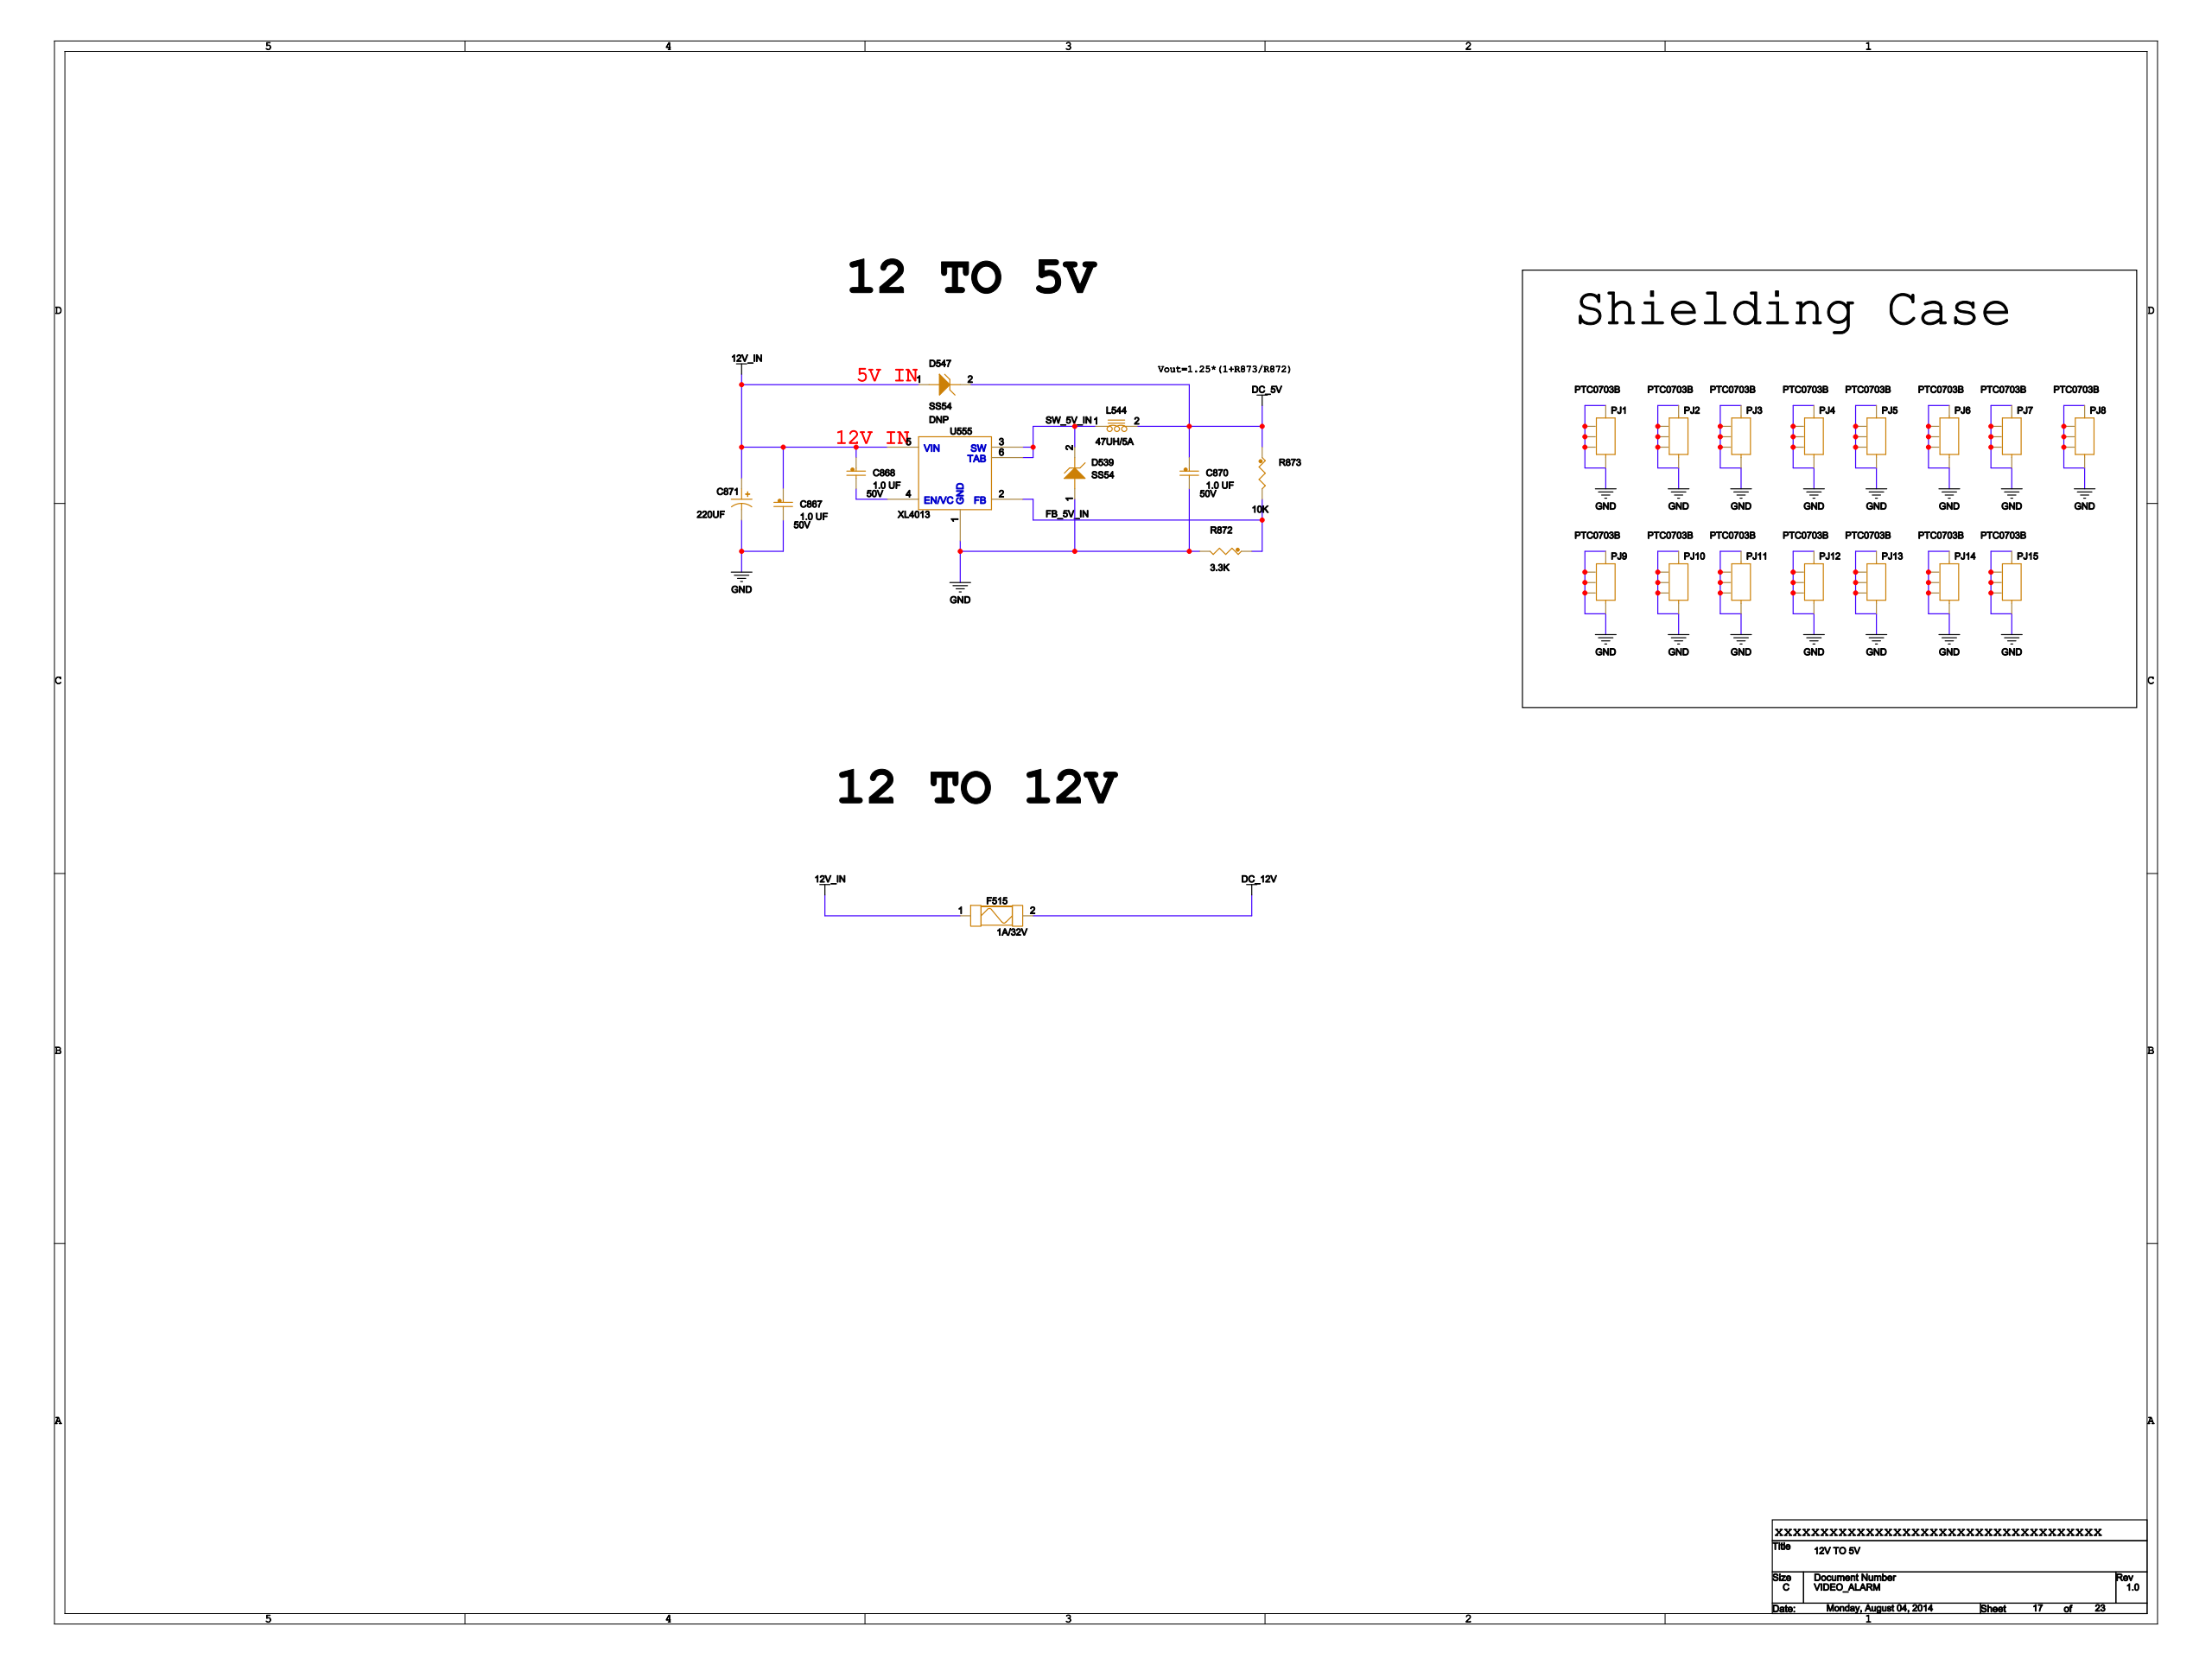Circuit board | Cadence Allegro | 994 parts | 728 nets | one sheet of the schematic
Parts on this sheet (reference | value | footprint):
C867 | 1.0 UF | 0603_CC
C868 | 1.0 UF | 0603_CC
C870 | 1.0 UF | 0603_CC
C871 | 220UF | CAPDIP0903
D539 | SS54 | DO-214AB
D547 | SS54 | DO-214AB
F515 | 1A/32V | 1206_CC
L544 | 47UH/5A | MT105
PJ1 | PTC0703B | PTC0703B_SMD
PJ2 | PTC0703B | PTC0703B_SMD
PJ3 | PTC0703B | PTC0703B_SMD
PJ4 | PTC0703B | PTC0703B_SMD
PJ5 | PTC0703B | PTC0703B_SMD
PJ6 | PTC0703B | PTC0703B_SMD
PJ7 | PTC0703B | PTC0703B_SMD
PJ8 | PTC0703B | PTC0703B_SMD
PJ9 | PTC0703B | PTC0703B_SMD
PJ10 | PTC0703B | PTC0703B_SMD
PJ11 | PTC0703B | PTC0703B_SMD
PJ12 | PTC0703B | PTC0703B_SMD
PJ13 | PTC0703B | PTC0703B_SMD
PJ14 | PTC0703B | PTC0703B_SMD
PJ15 | PTC0703B | PTC0703B_SMD
R872 | 3.3K | 0603_CC
R873 | 10K | 0603_CC
U555 | XL4013 | TO252-5L
Nets of these parts (net: part-pin ...):
GND: C867-2 C870-2 C871-2 D539-1 PJ1-1 PJ1-2 PJ1-3 PJ1-4 PJ1-5 PJ2-1 PJ2-2 PJ2-3 PJ2-4 PJ2-5 PJ3-1 PJ3-2 PJ3-3 PJ3-4 PJ3-5 PJ4-1 PJ4-2 PJ4-3 PJ4-4 PJ4-5 PJ5-1 PJ5-2 PJ5-3 PJ5-4 PJ5-5 PJ6-1 PJ6-2 PJ6-3 PJ6-4 PJ6-5 PJ7-1 PJ7-2 PJ7-3 PJ7-4 PJ7-5 PJ8-1 PJ8-2 PJ8-3 PJ8-4 PJ8-5 PJ9-1 PJ9-2 PJ9-3 PJ9-4 PJ9-5 PJ10-1 PJ10-2 PJ10-3 PJ10-4 PJ10-5 PJ11-1 PJ11-2 PJ11-3 PJ11-4 PJ11-5 PJ12-1 PJ12-2 PJ12-3 PJ12-4 PJ12-5 PJ13-1 PJ13-2 PJ13-3 PJ13-4 PJ13-5 PJ14-1 PJ14-2 PJ14-3 PJ14-4 PJ14-5 PJ15-1 PJ15-2 PJ15-3 PJ15-4 PJ15-5 R872-2 U555-1
FB_5V_IN: R872-1 R873-2 U555-2
SW_5V_IN: D539-2 L544-1 U555-3 U555-6
N22490042: C868-2 U555-4
12V_IN: C867-1 C868-1 C871-1 D547-1 F515-1 U555-5
DC_12V: F515-2
DC_5V: C870-1 D547-2 L544-2 R873-1